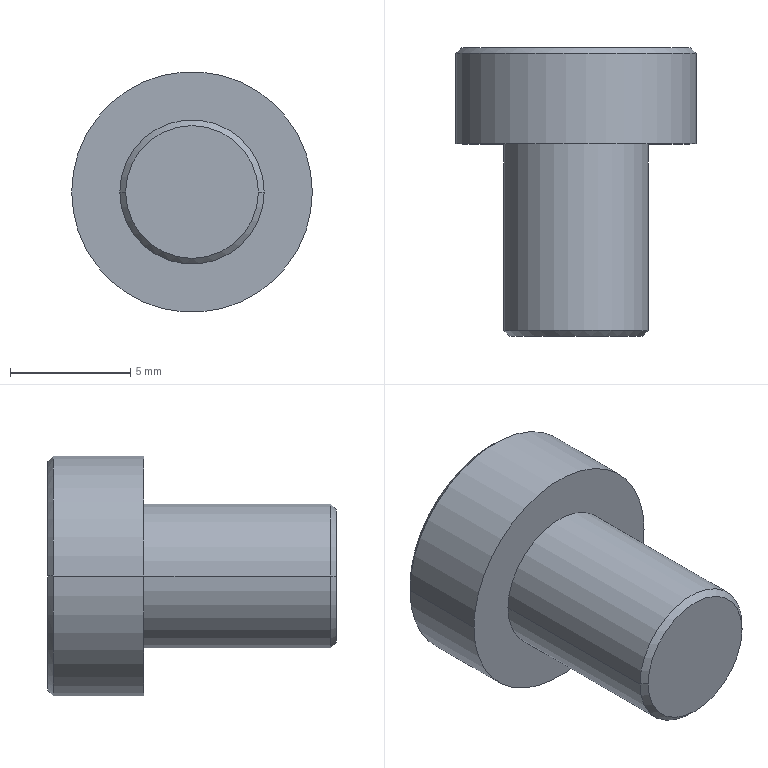Part | SolidWorks | features Chamfer 1, ICE 1, MoveCopyBody 1, Revolution 1 | 1 solid | 25 faces | box 10 x 12 x 10 mm | volume 492.529 mm3 | plane 15 | cone 6 | cylinder 4 | commonest cylinder face diameters 6 x2 10 x2
STEP:
#1=CARTESIAN_POINT('',(0.,6.345,0.));
#2=VERTEX_POINT('',#1);
#3=CARTESIAN_POINT('',(2.,7.5,0.));
#4=VERTEX_POINT('',#3);
#5=CARTESIAN_POINT('',(0.,6.345,0.));
#6=DIRECTION('',(0.866,0.5,0.));
#7=VECTOR('',#6,1000.);
#8=LINE('',#5,#7);
#9=EDGE_CURVE('',#2,#4,#8,.T.);
#10=ORIENTED_EDGE('',*,*,#9,.F.);
#11=CARTESIAN_POINT('',(-2.,7.5,0.));
#12=VERTEX_POINT('',#11);
#13=CARTESIAN_POINT('',(0.,6.345,0.));
#14=DIRECTION('',(-0.866,0.5,0.));
#15=VECTOR('',#14,1000.);
#16=LINE('',#13,#15);
#17=EDGE_CURVE('',#2,#12,#16,.T.);
#18=ORIENTED_EDGE('',*,*,#17,.T.);
#19=CARTESIAN_POINT('',(-1.732,7.5,1.));
#20=VERTEX_POINT('',#19);
#21=CARTESIAN_POINT('',(0.,7.5,0.));
#22=DIRECTION('',(0.,1.,0.));
#23=DIRECTION('',(1.,0.,0.));
#24=AXIS2_PLACEMENT_3D('',#21,#22,#23);
#25=CIRCLE('',#24,2.);
#26=EDGE_CURVE('',#12,#20,#25,.T.);
#27=ORIENTED_EDGE('',*,*,#26,.T.);
#28=CARTESIAN_POINT('',(0.,7.5,2.));
#29=VERTEX_POINT('',#28);
#30=CARTESIAN_POINT('',(0.,7.5,0.));
#31=DIRECTION('',(0.,1.,0.));
#32=DIRECTION('',(1.,0.,0.));
#33=AXIS2_PLACEMENT_3D('',#30,#31,#32);
#34=CIRCLE('',#33,2.);
#35=EDGE_CURVE('',#20,#29,#34,.T.);
#36=ORIENTED_EDGE('',*,*,#35,.T.);
#37=CARTESIAN_POINT('',(1.732,7.5,1.));
#38=VERTEX_POINT('',#37);
#39=CARTESIAN_POINT('',(0.,7.5,0.));
#40=DIRECTION('',(0.,1.,0.));
#41=DIRECTION('',(1.,0.,0.));
#42=AXIS2_PLACEMENT_3D('',#39,#40,#41);
#43=CIRCLE('',#42,2.);
#44=EDGE_CURVE('',#29,#38,#43,.T.);
#45=ORIENTED_EDGE('',*,*,#44,.T.);
#46=CARTESIAN_POINT('',(0.,7.5,0.));
#47=DIRECTION('',(0.,1.,0.));
#48=DIRECTION('',(1.,0.,0.));
#49=AXIS2_PLACEMENT_3D('',#46,#47,#48);
#50=CIRCLE('',#49,2.);
#51=EDGE_CURVE('',#38,#4,#50,.T.);
#52=ORIENTED_EDGE('',*,*,#51,.T.);
#53=EDGE_LOOP('',(#10,#18,#27,#36,#45,#52));
#54=FACE_OUTER_BOUND('',#53,.T.);
#55=CARTESIAN_POINT('',(0.,1006.345,0.));
#56=DIRECTION('',(0.,1.,0.));
#57=DIRECTION('',(1.,0.,0.));
#58=AXIS2_PLACEMENT_3D('',#55,#56,#57);
#59=CONICAL_SURFACE('',#58,1732.051,1.047);
#60=ADVANCED_FACE('',(#54),#59,.F.);
#61=CARTESIAN_POINT('',(-2.76,-1.5,0.));
#62=VERTEX_POINT('',#61);
#63=CARTESIAN_POINT('',(2.76,-1.5,0.));
#64=VERTEX_POINT('',#63);
#65=CARTESIAN_POINT('',(0.,-1.5,0.));
#66=DIRECTION('',(0.,-1.,0.));
#67=DIRECTION('',(-1.,0.,0.));
#68=AXIS2_PLACEMENT_3D('',#65,#66,#67);
#69=CIRCLE('',#68,2.76);
#70=EDGE_CURVE('',#62,#64,#69,.T.);
#71=ORIENTED_EDGE('',*,*,#70,.F.);
#72=CARTESIAN_POINT('',(-3.,-1.26,0.));
#73=VERTEX_POINT('',#72);
#74=CARTESIAN_POINT('',(-3.,-1.26,0.));
#75=DIRECTION('',(-0.7071,0.7071,0.));
#76=VECTOR('',#75,1000.);
#77=LINE('',#74,#76);
#78=EDGE_CURVE('',#62,#73,#77,.T.);
#79=ORIENTED_EDGE('',*,*,#78,.T.);
#80=CARTESIAN_POINT('',(3.,-1.26,0.));
#81=VERTEX_POINT('',#80);
#82=CARTESIAN_POINT('',(0.,-1.26,0.));
#83=DIRECTION('',(0.,1.,0.));
#84=DIRECTION('',(-1.,0.,0.));
#85=AXIS2_PLACEMENT_3D('',#82,#83,#84);
#86=CIRCLE('',#85,3.);
#87=EDGE_CURVE('',#81,#73,#86,.T.);
#88=ORIENTED_EDGE('',*,*,#87,.F.);
#89=CARTESIAN_POINT('',(3.,-1.26,0.));
#90=DIRECTION('',(0.7071,0.7071,0.));
#91=VECTOR('',#90,1000.);
#92=LINE('',#89,#91);
#93=EDGE_CURVE('',#64,#81,#92,.T.);
#94=ORIENTED_EDGE('',*,*,#93,.F.);
#95=EDGE_LOOP('',(#71,#79,#88,#94));
#96=FACE_OUTER_BOUND('',#95,.T.);
#97=CARTESIAN_POINT('',(0.,-1.26,0.));
#98=DIRECTION('',(0.,1.,0.));
#99=DIRECTION('',(1.,0.,0.));
#100=AXIS2_PLACEMENT_3D('',#97,#98,#99);
#101=CONICAL_SURFACE('',#100,3.,0.7854);
#102=ADVANCED_FACE('',(#96),#101,.T.);
#103=CARTESIAN_POINT('',(4.76,10.5,0.));
#104=VERTEX_POINT('',#103);
#105=CARTESIAN_POINT('',(-4.76,10.5,0.));
#106=VERTEX_POINT('',#105);
#107=CARTESIAN_POINT('',(0.,10.5,0.));
#108=DIRECTION('',(0.,1.,0.));
#109=DIRECTION('',(1.,0.,0.));
#110=AXIS2_PLACEMENT_3D('',#107,#108,#109);
#111=CIRCLE('',#110,4.76);
#112=EDGE_CURVE('',#104,#106,#111,.T.);
#113=ORIENTED_EDGE('',*,*,#112,.F.);
#114=CARTESIAN_POINT('',(5.,10.26,0.));
#115=VERTEX_POINT('',#114);
#116=CARTESIAN_POINT('',(4.76,10.5,0.));
#117=DIRECTION('',(0.7071,-0.7071,0.));
#118=VECTOR('',#117,1000.);
#119=LINE('',#116,#118);
#120=EDGE_CURVE('',#104,#115,#119,.T.);
#121=ORIENTED_EDGE('',*,*,#120,.T.);
#122=CARTESIAN_POINT('',(-5.,10.26,0.));
#123=VERTEX_POINT('',#122);
#124=CARTESIAN_POINT('',(0.,10.26,0.));
#125=DIRECTION('',(0.,-1.,0.));
#126=DIRECTION('',(1.,0.,0.));
#127=AXIS2_PLACEMENT_3D('',#124,#125,#126);
#128=CIRCLE('',#127,5.);
#129=EDGE_CURVE('',#123,#115,#128,.T.);
#130=ORIENTED_EDGE('',*,*,#129,.F.);
#131=CARTESIAN_POINT('',(-4.76,10.5,0.));
#132=DIRECTION('',(-0.7071,-0.7071,0.));
#133=VECTOR('',#132,1000.);
#134=LINE('',#131,#133);
#135=EDGE_CURVE('',#106,#123,#134,.T.);
#136=ORIENTED_EDGE('',*,*,#135,.F.);
#137=EDGE_LOOP('',(#113,#121,#130,#136));
#138=FACE_OUTER_BOUND('',#137,.T.);
#139=CARTESIAN_POINT('',(0.,10.5,0.));
#140=DIRECTION('',(0.,-1.,0.));
#141=DIRECTION('',(-1.,0.,0.));
#142=AXIS2_PLACEMENT_3D('',#139,#140,#141);
#143=CONICAL_SURFACE('',#142,4.76,0.7854);
#144=ADVANCED_FACE('',(#138),#143,.T.);
#145=CARTESIAN_POINT('',(5.,6.5,0.));
#146=VERTEX_POINT('',#145);
#147=CARTESIAN_POINT('',(-5.,6.5,0.));
#148=VERTEX_POINT('',#147);
#149=CARTESIAN_POINT('',(0.,6.5,0.));
#150=DIRECTION('',(0.,1.,0.));
#151=DIRECTION('',(1.,0.,0.));
#152=AXIS2_PLACEMENT_3D('',#149,#150,#151);
#153=CIRCLE('',#152,5.);
#154=EDGE_CURVE('',#146,#148,#153,.T.);
#155=ORIENTED_EDGE('',*,*,#154,.T.);
#156=CARTESIAN_POINT('',(-5.,6.345,0.));
#157=DIRECTION('',(0.,1.,0.));
#158=VECTOR('',#157,1000.);
#159=LINE('',#156,#158);
#160=EDGE_CURVE('',#148,#123,#159,.T.);
#161=ORIENTED_EDGE('',*,*,#160,.T.);
#162=ORIENTED_EDGE('',*,*,#129,.T.);
#163=CARTESIAN_POINT('',(5.,6.345,0.));
#164=DIRECTION('',(0.,1.,0.));
#165=VECTOR('',#164,1000.);
#166=LINE('',#163,#165);
#167=EDGE_CURVE('',#146,#115,#166,.T.);
#168=ORIENTED_EDGE('',*,*,#167,.F.);
#169=EDGE_LOOP('',(#155,#161,#162,#168));
#170=FACE_OUTER_BOUND('',#169,.T.);
#171=CARTESIAN_POINT('',(0.,6.345,0.));
#172=DIRECTION('',(0.,1.,0.));
#173=DIRECTION('',(1.,0.,0.));
#174=AXIS2_PLACEMENT_3D('',#171,#172,#173);
#175=CYLINDRICAL_SURFACE('',#174,5.);
#176=ADVANCED_FACE('',(#170),#175,.T.);
#177=ORIENTED_EDGE('',*,*,#87,.T.);
#178=CARTESIAN_POINT('',(-3.,6.5,0.));
#179=VERTEX_POINT('',#178);
#180=CARTESIAN_POINT('',(-3.,6.345,0.));
#181=DIRECTION('',(0.,1.,0.));
#182=VECTOR('',#181,1000.);
#183=LINE('',#180,#182);
#184=EDGE_CURVE('',#73,#179,#183,.T.);
#185=ORIENTED_EDGE('',*,*,#184,.T.);
#186=CARTESIAN_POINT('',(3.,6.5,0.));
#187=VERTEX_POINT('',#186);
#188=CARTESIAN_POINT('',(0.,6.5,0.));
#189=DIRECTION('',(0.,1.,0.));
#190=DIRECTION('',(1.,0.,0.));
#191=AXIS2_PLACEMENT_3D('',#188,#189,#190);
#192=CIRCLE('',#191,3.);
#193=EDGE_CURVE('',#187,#179,#192,.T.);
#194=ORIENTED_EDGE('',*,*,#193,.F.);
#195=CARTESIAN_POINT('',(3.,6.345,0.));
#196=DIRECTION('',(0.,1.,0.));
#197=VECTOR('',#196,1000.);
#198=LINE('',#195,#197);
#199=EDGE_CURVE('',#81,#187,#198,.T.);
#200=ORIENTED_EDGE('',*,*,#199,.F.);
#201=EDGE_LOOP('',(#177,#185,#194,#200));
#202=FACE_OUTER_BOUND('',#201,.T.);
#203=CARTESIAN_POINT('',(0.,6.345,0.));
#204=DIRECTION('',(0.,1.,0.));
#205=DIRECTION('',(1.,0.,0.));
#206=AXIS2_PLACEMENT_3D('',#203,#204,#205);
#207=CYLINDRICAL_SURFACE('',#206,3.);
#208=ADVANCED_FACE('',(#202),#207,.T.);
#209=CARTESIAN_POINT('',(1.155,10.5,2.));
#210=VERTEX_POINT('',#209);
#211=CARTESIAN_POINT('',(2.309,10.5,0.));
#212=VERTEX_POINT('',#211);
#213=CARTESIAN_POINT('',(1.155,10.5,2.));
#214=DIRECTION('',(0.5,0.,-0.866));
#215=VECTOR('',#214,1000.);
#216=LINE('',#213,#215);
#217=EDGE_CURVE('',#210,#212,#216,.T.);
#218=ORIENTED_EDGE('',*,*,#217,.F.);
#219=CARTESIAN_POINT('',(-1.155,10.5,2.));
#220=VERTEX_POINT('',#219);
#221=CARTESIAN_POINT('',(-1.155,10.5,2.));
#222=DIRECTION('',(1.,0.,0.));
#223=VECTOR('',#222,1000.);
#224=LINE('',#221,#223);
#225=EDGE_CURVE('',#220,#210,#224,.T.);
#226=ORIENTED_EDGE('',*,*,#225,.F.);
#227=CARTESIAN_POINT('',(-2.309,10.5,0.));
#228=VERTEX_POINT('',#227);
#229=CARTESIAN_POINT('',(-2.309,10.5,0.));
#230=DIRECTION('',(0.5,0.,0.866));
#231=VECTOR('',#230,1000.);
#232=LINE('',#229,#231);
#233=EDGE_CURVE('',#228,#220,#232,.T.);
#234=ORIENTED_EDGE('',*,*,#233,.F.);
#235=CARTESIAN_POINT('',(-1.155,10.5,-2.));
#236=VERTEX_POINT('',#235);
#237=CARTESIAN_POINT('',(-1.155,10.5,-2.));
#238=DIRECTION('',(-0.5,0.,0.866));
#239=VECTOR('',#238,1000.);
#240=LINE('',#237,#239);
#241=EDGE_CURVE('',#236,#228,#240,.T.);
#242=ORIENTED_EDGE('',*,*,#241,.F.);
#243=CARTESIAN_POINT('',(1.155,10.5,-2.));
#244=VERTEX_POINT('',#243);
#245=CARTESIAN_POINT('',(1.155,10.5,-2.));
#246=DIRECTION('',(-1.,0.,0.));
#247=VECTOR('',#246,1000.);
#248=LINE('',#245,#247);
#249=EDGE_CURVE('',#244,#236,#248,.T.);
#250=ORIENTED_EDGE('',*,*,#249,.F.);
#251=CARTESIAN_POINT('',(2.309,10.5,0.));
#252=DIRECTION('',(-0.5,0.,-0.866));
#253=VECTOR('',#252,1000.);
#254=LINE('',#251,#253);
#255=EDGE_CURVE('',#212,#244,#254,.T.);
#256=ORIENTED_EDGE('',*,*,#255,.F.);
#257=EDGE_LOOP('',(#218,#226,#234,#242,#250,#256));
#258=FACE_BOUND('',#257,.T.);
#259=CARTESIAN_POINT('',(0.,10.5,0.));
#260=DIRECTION('',(0.,1.,0.));
#261=DIRECTION('',(1.,0.,0.));
#262=AXIS2_PLACEMENT_3D('',#259,#260,#261);
#263=CIRCLE('',#262,4.76);
#264=EDGE_CURVE('',#106,#104,#263,.T.);
#265=ORIENTED_EDGE('',*,*,#264,.T.);
#266=ORIENTED_EDGE('',*,*,#112,.T.);
#267=EDGE_LOOP('',(#265,#266));
#268=FACE_OUTER_BOUND('',#267,.T.);
#269=CARTESIAN_POINT('',(-5.,10.5,0.));
#270=DIRECTION('',(0.,1.,0.));
#271=DIRECTION('',(1.,0.,0.));
#272=AXIS2_PLACEMENT_3D('',#269,#270,#271);
#273=PLANE('',#272);
#274=ADVANCED_FACE('',(#258,#268),#273,.T.);
#275=CARTESIAN_POINT('',(0.,-1.5,0.));
#276=DIRECTION('',(0.,-1.,0.));
#277=DIRECTION('',(-1.,0.,0.));
#278=AXIS2_PLACEMENT_3D('',#275,#276,#277);
#279=CIRCLE('',#278,2.76);
#280=EDGE_CURVE('',#64,#62,#279,.T.);
#281=ORIENTED_EDGE('',*,*,#280,.T.);
#282=ORIENTED_EDGE('',*,*,#70,.T.);
#283=EDGE_LOOP('',(#281,#282));
#284=FACE_OUTER_BOUND('',#283,.T.);
#285=CARTESIAN_POINT('',(-3.,-1.5,0.));
#286=DIRECTION('',(0.,-1.,0.));
#287=DIRECTION('',(-1.,0.,0.));
#288=AXIS2_PLACEMENT_3D('',#285,#286,#287);
#289=PLANE('',#288);
#290=ADVANCED_FACE('',(#284),#289,.T.);
#291=ORIENTED_EDGE('',*,*,#184,.F.);
#292=CARTESIAN_POINT('',(0.,-1.26,0.));
#293=DIRECTION('',(0.,1.,0.));
#294=DIRECTION('',(-1.,0.,0.));
#295=AXIS2_PLACEMENT_3D('',#292,#293,#294);
#296=CIRCLE('',#295,3.);
#297=EDGE_CURVE('',#73,#81,#296,.T.);
#298=ORIENTED_EDGE('',*,*,#297,.T.);
#299=ORIENTED_EDGE('',*,*,#199,.T.);
#300=CARTESIAN_POINT('',(0.,6.5,0.));
#301=DIRECTION('',(0.,1.,0.));
#302=DIRECTION('',(1.,0.,0.));
#303=AXIS2_PLACEMENT_3D('',#300,#301,#302);
#304=CIRCLE('',#303,3.);
#305=EDGE_CURVE('',#179,#187,#304,.T.);
#306=ORIENTED_EDGE('',*,*,#305,.F.);
#307=EDGE_LOOP('',(#291,#298,#299,#306));
#308=FACE_OUTER_BOUND('',#307,.T.);
#309=CARTESIAN_POINT('',(0.,6.345,0.));
#310=DIRECTION('',(0.,1.,0.));
#311=DIRECTION('',(1.,0.,0.));
#312=AXIS2_PLACEMENT_3D('',#309,#310,#311);
#313=CYLINDRICAL_SURFACE('',#312,3.);
#314=ADVANCED_FACE('',(#308),#313,.T.);
#315=ORIENTED_EDGE('',*,*,#193,.T.);
#316=ORIENTED_EDGE('',*,*,#305,.T.);
#317=EDGE_LOOP('',(#315,#316));
#318=FACE_BOUND('',#317,.T.);
#319=ORIENTED_EDGE('',*,*,#154,.F.);
#320=CARTESIAN_POINT('',(0.,6.5,0.));
#321=DIRECTION('',(0.,1.,0.));
#322=DIRECTION('',(1.,0.,0.));
#323=AXIS2_PLACEMENT_3D('',#320,#321,#322);
#324=CIRCLE('',#323,5.);
#325=EDGE_CURVE('',#148,#146,#324,.T.);
#326=ORIENTED_EDGE('',*,*,#325,.F.);
#327=EDGE_LOOP('',(#319,#326));
#328=FACE_OUTER_BOUND('',#327,.T.);
#329=CARTESIAN_POINT('',(-3.,6.5,0.));
#330=DIRECTION('',(0.,-1.,0.));
#331=DIRECTION('',(-1.,0.,0.));
#332=AXIS2_PLACEMENT_3D('',#329,#330,#331);
#333=PLANE('',#332);
#334=ADVANCED_FACE('',(#318,#328),#333,.T.);
#335=ORIENTED_EDGE('',*,*,#160,.F.);
#336=ORIENTED_EDGE('',*,*,#325,.T.);
#337=ORIENTED_EDGE('',*,*,#167,.T.);
#338=CARTESIAN_POINT('',(0.,10.26,0.));
#339=DIRECTION('',(0.,-1.,0.));
#340=DIRECTION('',(1.,0.,0.));
#341=AXIS2_PLACEMENT_3D('',#338,#339,#340);
#342=CIRCLE('',#341,5.);
#343=EDGE_CURVE('',#115,#123,#342,.T.);
#344=ORIENTED_EDGE('',*,*,#343,.T.);
#345=EDGE_LOOP('',(#335,#336,#337,#344));
#346=FACE_OUTER_BOUND('',#345,.T.);
#347=CARTESIAN_POINT('',(0.,6.345,0.));
#348=DIRECTION('',(0.,1.,0.));
#349=DIRECTION('',(1.,0.,0.));
#350=AXIS2_PLACEMENT_3D('',#347,#348,#349);
#351=CYLINDRICAL_SURFACE('',#350,5.);
#352=ADVANCED_FACE('',(#346),#351,.T.);
#353=ORIENTED_EDGE('',*,*,#120,.F.);
#354=ORIENTED_EDGE('',*,*,#264,.F.);
#355=ORIENTED_EDGE('',*,*,#135,.T.);
#356=ORIENTED_EDGE('',*,*,#343,.F.);
#357=EDGE_LOOP('',(#353,#354,#355,#356));
#358=FACE_OUTER_BOUND('',#357,.T.);
#359=CARTESIAN_POINT('',(0.,10.5,0.));
#360=DIRECTION('',(0.,-1.,0.));
#361=DIRECTION('',(-1.,0.,0.));
#362=AXIS2_PLACEMENT_3D('',#359,#360,#361);
#363=CONICAL_SURFACE('',#362,4.76,0.7854);
#364=ADVANCED_FACE('',(#358),#363,.T.);
#365=ORIENTED_EDGE('',*,*,#78,.F.);
#366=ORIENTED_EDGE('',*,*,#280,.F.);
#367=ORIENTED_EDGE('',*,*,#93,.T.);
#368=ORIENTED_EDGE('',*,*,#297,.F.);
#369=EDGE_LOOP('',(#365,#366,#367,#368));
#370=FACE_OUTER_BOUND('',#369,.T.);
#371=CARTESIAN_POINT('',(0.,-1.26,0.));
#372=DIRECTION('',(0.,1.,0.));
#373=DIRECTION('',(1.,0.,0.));
#374=AXIS2_PLACEMENT_3D('',#371,#372,#373);
#375=CONICAL_SURFACE('',#374,3.,0.7854);
#376=ADVANCED_FACE('',(#370),#375,.T.);
#377=CARTESIAN_POINT('',(1.155,7.5,-2.));
#378=VERTEX_POINT('',#377);
#379=CARTESIAN_POINT('',(0.,7.5,-2.));
#380=VERTEX_POINT('',#379);
#381=CARTESIAN_POINT('',(1.155,7.5,-2.));
#382=DIRECTION('',(-1.,0.,0.));
#383=VECTOR('',#382,1000.);
#384=LINE('',#381,#383);
#385=EDGE_CURVE('',#378,#380,#384,.T.);
#386=ORIENTED_EDGE('',*,*,#385,.F.);
#387=CARTESIAN_POINT('',(1.155,7.5,-2.));
#388=DIRECTION('',(0.,1.,0.));
#389=VECTOR('',#388,1000.);
#390=LINE('',#387,#389);
#391=EDGE_CURVE('',#378,#244,#390,.T.);
#392=ORIENTED_EDGE('',*,*,#391,.T.);
#393=ORIENTED_EDGE('',*,*,#249,.T.);
#394=CARTESIAN_POINT('',(-1.155,7.5,-2.));
#395=VERTEX_POINT('',#394);
#396=CARTESIAN_POINT('',(-1.155,7.5,-2.));
#397=DIRECTION('',(0.,1.,0.));
#398=VECTOR('',#397,1000.);
#399=LINE('',#396,#398);
#400=EDGE_CURVE('',#395,#236,#399,.T.);
#401=ORIENTED_EDGE('',*,*,#400,.F.);
#402=CARTESIAN_POINT('',(1.155,7.5,-2.));
#403=DIRECTION('',(-1.,0.,0.));
#404=VECTOR('',#403,1000.);
#405=LINE('',#402,#404);
#406=EDGE_CURVE('',#380,#395,#405,.T.);
#407=ORIENTED_EDGE('',*,*,#406,.F.);
#408=EDGE_LOOP('',(#386,#392,#393,#401,#407));
#409=FACE_OUTER_BOUND('',#408,.T.);
#410=CARTESIAN_POINT('',(1.155,7.5,-2.));
#411=DIRECTION('',(0.,0.,-1.));
#412=DIRECTION('',(1.,0.,0.));
#413=AXIS2_PLACEMENT_3D('',#410,#411,#412);
#414=PLANE('',#413);
#415=ADVANCED_FACE('',(#409),#414,.F.);
#416=CARTESIAN_POINT('',(2.309,7.5,0.));
#417=VERTEX_POINT('',#416);
#418=CARTESIAN_POINT('',(1.732,7.5,-1.));
#419=VERTEX_POINT('',#418);
#420=CARTESIAN_POINT('',(2.309,7.5,0.));
#421=DIRECTION('',(-0.5,0.,-0.866));
#422=VECTOR('',#421,1000.);
#423=LINE('',#420,#422);
#424=EDGE_CURVE('',#417,#419,#423,.T.);
#425=ORIENTED_EDGE('',*,*,#424,.F.);
#426=CARTESIAN_POINT('',(2.309,7.5,0.));
#427=DIRECTION('',(0.,1.,0.));
#428=VECTOR('',#427,1000.);
#429=LINE('',#426,#428);
#430=EDGE_CURVE('',#417,#212,#429,.T.);
#431=ORIENTED_EDGE('',*,*,#430,.T.);
#432=ORIENTED_EDGE('',*,*,#255,.T.);
#433=ORIENTED_EDGE('',*,*,#391,.F.);
#434=CARTESIAN_POINT('',(2.309,7.5,0.));
#435=DIRECTION('',(-0.5,0.,-0.866));
#436=VECTOR('',#435,1000.);
#437=LINE('',#434,#436);
#438=EDGE_CURVE('',#419,#378,#437,.T.);
#439=ORIENTED_EDGE('',*,*,#438,.F.);
#440=EDGE_LOOP('',(#425,#431,#432,#433,#439));
#441=FACE_OUTER_BOUND('',#440,.T.);
#442=CARTESIAN_POINT('',(2.309,7.5,0.));
#443=DIRECTION('',(0.866,0.,-0.5));
#444=DIRECTION('',(0.5,0.,0.866));
#445=AXIS2_PLACEMENT_3D('',#442,#443,#444);
#446=PLANE('',#445);
#447=ADVANCED_FACE('',(#441),#446,.F.);
#448=CARTESIAN_POINT('',(1.155,7.5,2.));
#449=VERTEX_POINT('',#448);
#450=CARTESIAN_POINT('',(1.155,7.5,2.));
#451=DIRECTION('',(0.5,0.,-0.866));
#452=VECTOR('',#451,1000.);
#453=LINE('',#450,#452);
#454=EDGE_CURVE('',#449,#38,#453,.T.);
#455=ORIENTED_EDGE('',*,*,#454,.F.);
#456=CARTESIAN_POINT('',(1.155,7.5,2.));
#457=DIRECTION('',(0.,1.,0.));
#458=VECTOR('',#457,1000.);
#459=LINE('',#456,#458);
#460=EDGE_CURVE('',#449,#210,#459,.T.);
#461=ORIENTED_EDGE('',*,*,#460,.T.);
#462=ORIENTED_EDGE('',*,*,#217,.T.);
#463=ORIENTED_EDGE('',*,*,#430,.F.);
#464=CARTESIAN_POINT('',(1.155,7.5,2.));
#465=DIRECTION('',(0.5,0.,-0.866));
#466=VECTOR('',#465,1000.);
#467=LINE('',#464,#466);
#468=EDGE_CURVE('',#38,#417,#467,.T.);
#469=ORIENTED_EDGE('',*,*,#468,.F.);
#470=EDGE_LOOP('',(#455,#461,#462,#463,#469));
#471=FACE_OUTER_BOUND('',#470,.T.);
#472=CARTESIAN_POINT('',(1.155,7.5,2.));
#473=DIRECTION('',(0.866,0.,0.5));
#474=DIRECTION('',(-0.5,0.,0.866));
#475=AXIS2_PLACEMENT_3D('',#472,#473,#474);
#476=PLANE('',#475);
#477=ADVANCED_FACE('',(#471),#476,.F.);
#478=CARTESIAN_POINT('',(-1.155,7.5,2.));
#479=VERTEX_POINT('',#478);
#480=CARTESIAN_POINT('',(-1.155,7.5,2.));
#481=DIRECTION('',(1.,0.,0.));
#482=VECTOR('',#481,1000.);
#483=LINE('',#480,#482);
#484=EDGE_CURVE('',#479,#29,#483,.T.);
#485=ORIENTED_EDGE('',*,*,#484,.F.);
#486=CARTESIAN_POINT('',(-1.155,7.5,2.));
#487=DIRECTION('',(0.,1.,0.));
#488=VECTOR('',#487,1000.);
#489=LINE('',#486,#488);
#490=EDGE_CURVE('',#479,#220,#489,.T.);
#491=ORIENTED_EDGE('',*,*,#490,.T.);
#492=ORIENTED_EDGE('',*,*,#225,.T.);
#493=ORIENTED_EDGE('',*,*,#460,.F.);
#494=CARTESIAN_POINT('',(-1.155,7.5,2.));
#495=DIRECTION('',(1.,0.,0.));
#496=VECTOR('',#495,1000.);
#497=LINE('',#494,#496);
#498=EDGE_CURVE('',#29,#449,#497,.T.);
#499=ORIENTED_EDGE('',*,*,#498,.F.);
#500=EDGE_LOOP('',(#485,#491,#492,#493,#499));
#501=FACE_OUTER_BOUND('',#500,.T.);
#502=CARTESIAN_POINT('',(-1.155,7.5,2.));
#503=DIRECTION('',(0.,0.,1.));
#504=DIRECTION('',(-1.,0.,0.));
#505=AXIS2_PLACEMENT_3D('',#502,#503,#504);
#506=PLANE('',#505);
#507=ADVANCED_FACE('',(#501),#506,.F.);
#508=CARTESIAN_POINT('',(-2.309,7.5,0.));
#509=VERTEX_POINT('',#508);
#510=CARTESIAN_POINT('',(-2.309,7.5,0.));
#511=DIRECTION('',(0.5,0.,0.866));
#512=VECTOR('',#511,1000.);
#513=LINE('',#510,#512);
#514=EDGE_CURVE('',#509,#20,#513,.T.);
#515=ORIENTED_EDGE('',*,*,#514,.F.);
#516=CARTESIAN_POINT('',(-2.309,7.5,0.));
#517=DIRECTION('',(0.,1.,0.));
#518=VECTOR('',#517,1000.);
#519=LINE('',#516,#518);
#520=EDGE_CURVE('',#509,#228,#519,.T.);
#521=ORIENTED_EDGE('',*,*,#520,.T.);
#522=ORIENTED_EDGE('',*,*,#233,.T.);
#523=ORIENTED_EDGE('',*,*,#490,.F.);
#524=CARTESIAN_POINT('',(-2.309,7.5,0.));
#525=DIRECTION('',(0.5,0.,0.866));
#526=VECTOR('',#525,1000.);
#527=LINE('',#524,#526);
#528=EDGE_CURVE('',#20,#479,#527,.T.);
#529=ORIENTED_EDGE('',*,*,#528,.F.);
#530=EDGE_LOOP('',(#515,#521,#522,#523,#529));
#531=FACE_OUTER_BOUND('',#530,.T.);
#532=CARTESIAN_POINT('',(-2.309,7.5,0.));
#533=DIRECTION('',(-0.866,0.,0.5));
#534=DIRECTION('',(-0.5,0.,-0.866));
#535=AXIS2_PLACEMENT_3D('',#532,#533,#534);
#536=PLANE('',#535);
#537=ADVANCED_FACE('',(#531),#536,.F.);
#538=CARTESIAN_POINT('',(-1.732,7.5,-1.));
#539=VERTEX_POINT('',#538);
#540=CARTESIAN_POINT('',(-1.155,7.5,-2.));
#541=DIRECTION('',(-0.5,0.,0.866));
#542=VECTOR('',#541,1000.);
#543=LINE('',#540,#542);
#544=EDGE_CURVE('',#395,#539,#543,.T.);
#545=ORIENTED_EDGE('',*,*,#544,.F.);
#546=ORIENTED_EDGE('',*,*,#400,.T.);
#547=ORIENTED_EDGE('',*,*,#241,.T.);
#548=ORIENTED_EDGE('',*,*,#520,.F.);
#549=CARTESIAN_POINT('',(-1.155,7.5,-2.));
#550=DIRECTION('',(-0.5,0.,0.866));
#551=VECTOR('',#550,1000.);
#552=LINE('',#549,#551);
#553=EDGE_CURVE('',#539,#509,#552,.T.);
#554=ORIENTED_EDGE('',*,*,#553,.F.);
#555=EDGE_LOOP('',(#545,#546,#547,#548,#554));
#556=FACE_OUTER_BOUND('',#555,.T.);
#557=CARTESIAN_POINT('',(-1.155,7.5,-2.));
#558=DIRECTION('',(-0.866,0.,-0.5));
#559=DIRECTION('',(0.5,0.,-0.866));
#560=AXIS2_PLACEMENT_3D('',#557,#558,#559);
#561=PLANE('',#560);
#562=ADVANCED_FACE('',(#556),#561,.F.);
#563=ORIENTED_EDGE('',*,*,#498,.T.);
#564=ORIENTED_EDGE('',*,*,#454,.T.);
#565=ORIENTED_EDGE('',*,*,#44,.F.);
#566=EDGE_LOOP('',(#563,#564,#565));
#567=FACE_OUTER_BOUND('',#566,.T.);
#568=CARTESIAN_POINT('',(-1.155,7.5,-2.));
#569=DIRECTION('',(0.,1.,0.));
#570=DIRECTION('',(0.,0.,1.));
#571=AXIS2_PLACEMENT_3D('',#568,#569,#570);
#572=PLANE('',#571);
#573=ADVANCED_FACE('',(#567),#572,.T.);
#574=ORIENTED_EDGE('',*,*,#468,.T.);
#575=ORIENTED_EDGE('',*,*,#424,.T.);
#576=CARTESIAN_POINT('',(0.,7.5,0.));
#577=DIRECTION('',(0.,1.,0.));
#578=DIRECTION('',(1.,0.,0.));
#579=AXIS2_PLACEMENT_3D('',#576,#577,#578);
#580=CIRCLE('',#579,2.);
#581=EDGE_CURVE('',#4,#419,#580,.T.);
#582=ORIENTED_EDGE('',*,*,#581,.F.);
#583=ORIENTED_EDGE('',*,*,#51,.F.);
#584=EDGE_LOOP('',(#574,#575,#582,#583));
#585=FACE_OUTER_BOUND('',#584,.T.);
#586=CARTESIAN_POINT('',(-1.155,7.5,-2.));
#587=DIRECTION('',(0.,1.,0.));
#588=DIRECTION('',(0.,0.,1.));
#589=AXIS2_PLACEMENT_3D('',#586,#587,#588);
#590=PLANE('',#589);
#591=ADVANCED_FACE('',(#585),#590,.T.);
#592=ORIENTED_EDGE('',*,*,#438,.T.);
#593=ORIENTED_EDGE('',*,*,#385,.T.);
#594=CARTESIAN_POINT('',(0.,7.5,0.));
#595=DIRECTION('',(0.,1.,0.));
#596=DIRECTION('',(1.,0.,0.));
#597=AXIS2_PLACEMENT_3D('',#594,#595,#596);
#598=CIRCLE('',#597,2.);
#599=EDGE_CURVE('',#419,#380,#598,.T.);
#600=ORIENTED_EDGE('',*,*,#599,.F.);
#601=EDGE_LOOP('',(#592,#593,#600));
#602=FACE_OUTER_BOUND('',#601,.T.);
#603=CARTESIAN_POINT('',(-1.155,7.5,-2.));
#604=DIRECTION('',(0.,1.,0.));
#605=DIRECTION('',(0.,0.,1.));
#606=AXIS2_PLACEMENT_3D('',#603,#604,#605);
#607=PLANE('',#606);
#608=ADVANCED_FACE('',(#602),#607,.T.);
#609=ORIENTED_EDGE('',*,*,#406,.T.);
#610=ORIENTED_EDGE('',*,*,#544,.T.);
#611=CARTESIAN_POINT('',(0.,7.5,0.));
#612=DIRECTION('',(0.,1.,0.));
#613=DIRECTION('',(1.,0.,0.));
#614=AXIS2_PLACEMENT_3D('',#611,#612,#613);
#615=CIRCLE('',#614,2.);
#616=EDGE_CURVE('',#380,#539,#615,.T.);
#617=ORIENTED_EDGE('',*,*,#616,.F.);
#618=EDGE_LOOP('',(#609,#610,#617));
#619=FACE_OUTER_BOUND('',#618,.T.);
#620=CARTESIAN_POINT('',(-1.155,7.5,-2.));
#621=DIRECTION('',(0.,1.,0.));
#622=DIRECTION('',(0.,0.,1.));
#623=AXIS2_PLACEMENT_3D('',#620,#621,#622);
#624=PLANE('',#623);
#625=ADVANCED_FACE('',(#619),#624,.T.);
#626=ORIENTED_EDGE('',*,*,#553,.T.);
#627=ORIENTED_EDGE('',*,*,#514,.T.);
#628=ORIENTED_EDGE('',*,*,#26,.F.);
#629=CARTESIAN_POINT('',(0.,7.5,0.));
#630=DIRECTION('',(0.,1.,0.));
#631=DIRECTION('',(1.,0.,0.));
#632=AXIS2_PLACEMENT_3D('',#629,#630,#631);
#633=CIRCLE('',#632,2.);
#634=EDGE_CURVE('',#539,#12,#633,.T.);
#635=ORIENTED_EDGE('',*,*,#634,.F.);
#636=EDGE_LOOP('',(#626,#627,#628,#635));
#637=FACE_OUTER_BOUND('',#636,.T.);
#638=CARTESIAN_POINT('',(-1.155,7.5,-2.));
#639=DIRECTION('',(0.,1.,0.));
#640=DIRECTION('',(0.,0.,1.));
#641=AXIS2_PLACEMENT_3D('',#638,#639,#640);
#642=PLANE('',#641);
#643=ADVANCED_FACE('',(#637),#642,.T.);
#644=ORIENTED_EDGE('',*,*,#528,.T.);
#645=ORIENTED_EDGE('',*,*,#484,.T.);
#646=ORIENTED_EDGE('',*,*,#35,.F.);
#647=EDGE_LOOP('',(#644,#645,#646));
#648=FACE_OUTER_BOUND('',#647,.T.);
#649=CARTESIAN_POINT('',(-1.155,7.5,-2.));
#650=DIRECTION('',(0.,1.,0.));
#651=DIRECTION('',(0.,0.,1.));
#652=AXIS2_PLACEMENT_3D('',#649,#650,#651);
#653=PLANE('',#652);
#654=ADVANCED_FACE('',(#648),#653,.T.);
#655=ORIENTED_EDGE('',*,*,#17,.F.);
#656=ORIENTED_EDGE('',*,*,#9,.T.);
#657=ORIENTED_EDGE('',*,*,#581,.T.);
#658=ORIENTED_EDGE('',*,*,#599,.T.);
#659=ORIENTED_EDGE('',*,*,#616,.T.);
#660=ORIENTED_EDGE('',*,*,#634,.T.);
#661=EDGE_LOOP('',(#655,#656,#657,#658,#659,#660));
#662=FACE_OUTER_BOUND('',#661,.T.);
#663=CARTESIAN_POINT('',(0.,1006.345,0.));
#664=DIRECTION('',(0.,1.,0.));
#665=DIRECTION('',(1.,0.,0.));
#666=AXIS2_PLACEMENT_3D('',#663,#664,#665);
#667=CONICAL_SURFACE('',#666,1732.051,1.047);
#668=ADVANCED_FACE('',(#662),#667,.F.);
#669=CLOSED_SHELL('',(#60,#102,#144,#176,#208,#274,#290,#314,#334,#352,#364,#376,#415,#447,#477,#507,#537,#562,#573,#591,#608,#625,#643,#654,#668));
#670=MANIFOLD_SOLID_BREP('',#669);
#671=CARTESIAN_POINT('',(0.,0.,0.));
#672=DIRECTION('',(0.,0.,1.));
#673=DIRECTION('',(1.,0.,0.));
#674=AXIS2_PLACEMENT_3D('',#671,#672,#673);
#675=(LENGTH_UNIT()NAMED_UNIT(*)SI_UNIT(.MILLI.,.METRE.));
#676=UNCERTAINTY_MEASURE_WITH_UNIT(LENGTH_MEASURE(0.00001),#675,'','');
#677=(NAMED_UNIT(*)PLANE_ANGLE_UNIT()SI_UNIT($,.RADIAN.));
#678=(NAMED_UNIT(*)SI_UNIT($,.STERADIAN.)SOLID_ANGLE_UNIT());
#679=(GEOMETRIC_REPRESENTATION_CONTEXT(3)GLOBAL_UNCERTAINTY_ASSIGNED_CONTEXT((#676))GLOBAL_UNIT_ASSIGNED_CONTEXT((#675,#677,#678))REPRESENTATION_CONTEXT('',''));
#680=ADVANCED_BREP_SHAPE_REPRESENTATION('',(#670,#674),#679);